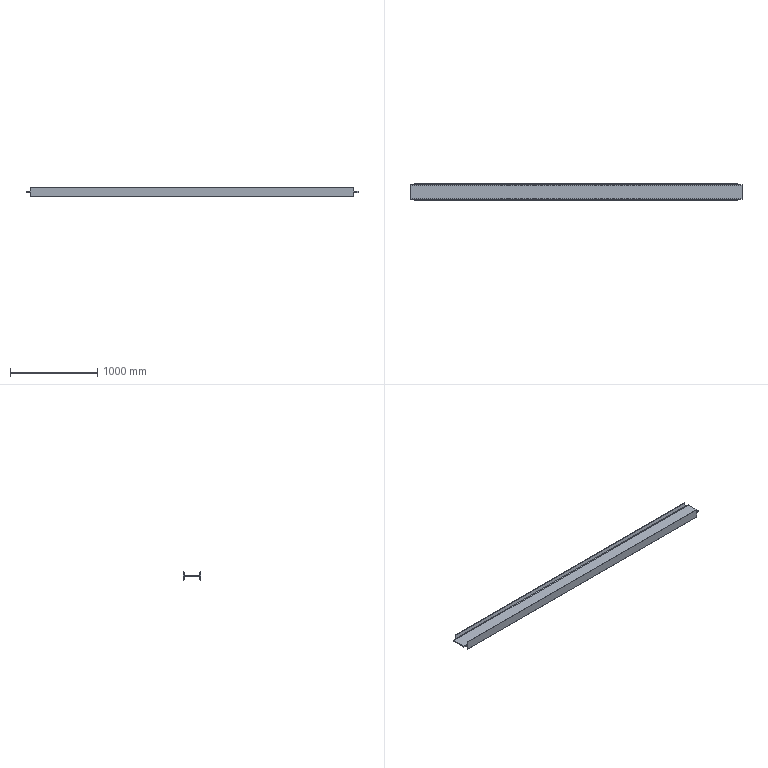Part | SolidWorks | features Fillet 2, ICE 2, Extrusion 1 | 1 solid | 30 faces | box 3800 x 200 x 102 mm | volume 14290911 mm3 | plane 22 | cylinder 8 | commonest cylinder face diameters 9 x4 18 x4
STEP:
#1=CARTESIAN_POINT('',(0.,15.,8.033));
#2=VERTEX_POINT('',#1);
#3=CARTESIAN_POINT('',(0.,15.,-8.033));
#4=VERTEX_POINT('',#3);
#5=CARTESIAN_POINT('',(0.,15.,51.));
#6=DIRECTION('',(0.,0.,-1.));
#7=VECTOR('',#6,1000.);
#8=LINE('',#5,#7);
#9=EDGE_CURVE('',#2,#4,#8,.T.);
#10=ORIENTED_EDGE('',*,*,#9,.F.);
#11=CARTESIAN_POINT('',(0.,22.149,4.5));
#12=VERTEX_POINT('',#11);
#13=CARTESIAN_POINT('',(0.,22.149,13.5));
#14=DIRECTION('',(1.,0.,0.));
#15=DIRECTION('',(0.,0.,-1.));
#16=AXIS2_PLACEMENT_3D('',#13,#14,#15);
#17=CIRCLE('',#16,9.);
#18=EDGE_CURVE('',#2,#12,#17,.T.);
#19=ORIENTED_EDGE('',*,*,#18,.T.);
#20=CARTESIAN_POINT('',(0.,177.851,4.5));
#21=VERTEX_POINT('',#20);
#22=CARTESIAN_POINT('',(0.,185.475,4.5));
#23=DIRECTION('',(0.,-1.,0.));
#24=VECTOR('',#23,1000.);
#25=LINE('',#22,#24);
#26=EDGE_CURVE('',#21,#12,#25,.T.);
#27=ORIENTED_EDGE('',*,*,#26,.F.);
#28=CARTESIAN_POINT('',(0.,185.,8.033));
#29=VERTEX_POINT('',#28);
#30=CARTESIAN_POINT('',(0.,177.851,13.5));
#31=DIRECTION('',(1.,0.,0.));
#32=DIRECTION('',(0.,0.,-1.));
#33=AXIS2_PLACEMENT_3D('',#30,#31,#32);
#34=CIRCLE('',#33,9.);
#35=EDGE_CURVE('',#21,#29,#34,.T.);
#36=ORIENTED_EDGE('',*,*,#35,.T.);
#37=CARTESIAN_POINT('',(0.,185.,-8.033));
#38=VERTEX_POINT('',#37);
#39=CARTESIAN_POINT('',(0.,185.,51.));
#40=DIRECTION('',(0.,0.,1.));
#41=VECTOR('',#40,1000.);
#42=LINE('',#39,#41);
#43=EDGE_CURVE('',#38,#29,#42,.T.);
#44=ORIENTED_EDGE('',*,*,#43,.F.);
#45=CARTESIAN_POINT('',(0.,177.851,-4.5));
#46=VERTEX_POINT('',#45);
#47=CARTESIAN_POINT('',(0.,177.851,-13.5));
#48=DIRECTION('',(1.,0.,0.));
#49=DIRECTION('',(0.,0.,-1.));
#50=AXIS2_PLACEMENT_3D('',#47,#48,#49);
#51=CIRCLE('',#50,9.);
#52=EDGE_CURVE('',#38,#46,#51,.T.);
#53=ORIENTED_EDGE('',*,*,#52,.T.);
#54=CARTESIAN_POINT('',(0.,22.149,-4.5));
#55=VERTEX_POINT('',#54);
#56=CARTESIAN_POINT('',(0.,185.475,-4.5));
#57=DIRECTION('',(0.,1.,0.));
#58=VECTOR('',#57,1000.);
#59=LINE('',#56,#58);
#60=EDGE_CURVE('',#55,#46,#59,.T.);
#61=ORIENTED_EDGE('',*,*,#60,.F.);
#62=CARTESIAN_POINT('',(0.,22.149,-13.5));
#63=DIRECTION('',(1.,0.,0.));
#64=DIRECTION('',(0.,0.,-1.));
#65=AXIS2_PLACEMENT_3D('',#62,#63,#64);
#66=CIRCLE('',#65,9.);
#67=EDGE_CURVE('',#55,#4,#66,.T.);
#68=ORIENTED_EDGE('',*,*,#67,.T.);
#69=EDGE_LOOP('',(#10,#19,#27,#36,#44,#53,#61,#68));
#70=FACE_OUTER_BOUND('',#69,.T.);
#71=CARTESIAN_POINT('',(0.,200.,51.));
#72=DIRECTION('',(1.,0.,0.));
#73=DIRECTION('',(0.,0.,-1.));
#74=AXIS2_PLACEMENT_3D('',#71,#72,#73);
#75=PLANE('',#74);
#76=ADVANCED_FACE('',(#70),#75,.F.);
#77=CARTESIAN_POINT('',(3753.5,2.963,51.));
#78=VERTEX_POINT('',#77);
#79=CARTESIAN_POINT('',(46.5,2.963,51.));
#80=VERTEX_POINT('',#79);
#81=CARTESIAN_POINT('',(3800.,2.963,51.));
#82=DIRECTION('',(-1.,0.,0.));
#83=VECTOR('',#82,1000.);
#84=LINE('',#81,#83);
#85=EDGE_CURVE('',#78,#80,#84,.T.);
#86=ORIENTED_EDGE('',*,*,#85,.T.);
#87=CARTESIAN_POINT('',(46.5,0.,51.));
#88=VERTEX_POINT('',#87);
#89=CARTESIAN_POINT('',(46.5,15.,51.));
#90=DIRECTION('',(0.,-1.,0.));
#91=VECTOR('',#90,1000.);
#92=LINE('',#89,#91);
#93=EDGE_CURVE('',#80,#88,#92,.T.);
#94=ORIENTED_EDGE('',*,*,#93,.T.);
#95=CARTESIAN_POINT('',(3753.5,0.,51.));
#96=VERTEX_POINT('',#95);
#97=CARTESIAN_POINT('',(3800.,0.,51.));
#98=DIRECTION('',(-1.,0.,0.));
#99=VECTOR('',#98,1000.);
#100=LINE('',#97,#99);
#101=EDGE_CURVE('',#96,#88,#100,.T.);
#102=ORIENTED_EDGE('',*,*,#101,.F.);
#103=CARTESIAN_POINT('',(3753.5,15.,51.));
#104=DIRECTION('',(0.,-1.,0.));
#105=VECTOR('',#104,1000.);
#106=LINE('',#103,#105);
#107=EDGE_CURVE('',#78,#96,#106,.T.);
#108=ORIENTED_EDGE('',*,*,#107,.F.);
#109=EDGE_LOOP('',(#86,#94,#102,#108));
#110=FACE_OUTER_BOUND('',#109,.T.);
#111=CARTESIAN_POINT('',(3800.,6.775,51.));
#112=DIRECTION('',(0.,0.,-1.));
#113=DIRECTION('',(-1.,0.,0.));
#114=AXIS2_PLACEMENT_3D('',#111,#112,#113);
#115=PLANE('',#114);
#116=ADVANCED_FACE('',(#110),#115,.F.);
#117=ORIENTED_EDGE('',*,*,#101,.T.);
#118=CARTESIAN_POINT('',(46.5,0.,-51.));
#119=VERTEX_POINT('',#118);
#120=CARTESIAN_POINT('',(46.5,0.,51.));
#121=DIRECTION('',(0.,0.,1.));
#122=VECTOR('',#121,1000.);
#123=LINE('',#120,#122);
#124=EDGE_CURVE('',#119,#88,#123,.T.);
#125=ORIENTED_EDGE('',*,*,#124,.F.);
#126=CARTESIAN_POINT('',(3753.5,0.,-51.));
#127=VERTEX_POINT('',#126);
#128=CARTESIAN_POINT('',(3800.,0.,-51.));
#129=DIRECTION('',(-1.,0.,0.));
#130=VECTOR('',#129,1000.);
#131=LINE('',#128,#130);
#132=EDGE_CURVE('',#127,#119,#131,.T.);
#133=ORIENTED_EDGE('',*,*,#132,.F.);
#134=CARTESIAN_POINT('',(3753.5,0.,51.));
#135=DIRECTION('',(0.,0.,-1.));
#136=VECTOR('',#135,1000.);
#137=LINE('',#134,#136);
#138=EDGE_CURVE('',#96,#127,#137,.T.);
#139=ORIENTED_EDGE('',*,*,#138,.F.);
#140=EDGE_LOOP('',(#117,#125,#133,#139));
#141=FACE_OUTER_BOUND('',#140,.T.);
#142=CARTESIAN_POINT('',(3800.,0.,51.));
#143=DIRECTION('',(0.,1.,0.));
#144=DIRECTION('',(0.,0.,1.));
#145=AXIS2_PLACEMENT_3D('',#142,#143,#144);
#146=PLANE('',#145);
#147=ADVANCED_FACE('',(#141),#146,.F.);
#148=ORIENTED_EDGE('',*,*,#132,.T.);
#149=CARTESIAN_POINT('',(46.5,2.963,-51.));
#150=VERTEX_POINT('',#149);
#151=CARTESIAN_POINT('',(46.5,15.,-51.));
#152=DIRECTION('',(0.,-1.,0.));
#153=VECTOR('',#152,1000.);
#154=LINE('',#151,#153);
#155=EDGE_CURVE('',#150,#119,#154,.T.);
#156=ORIENTED_EDGE('',*,*,#155,.F.);
#157=CARTESIAN_POINT('',(3753.5,2.963,-51.));
#158=VERTEX_POINT('',#157);
#159=CARTESIAN_POINT('',(3800.,2.963,-51.));
#160=DIRECTION('',(1.,0.,0.));
#161=VECTOR('',#160,1000.);
#162=LINE('',#159,#161);
#163=EDGE_CURVE('',#150,#158,#162,.T.);
#164=ORIENTED_EDGE('',*,*,#163,.T.);
#165=CARTESIAN_POINT('',(3753.5,15.,-51.));
#166=DIRECTION('',(0.,-1.,0.));
#167=VECTOR('',#166,1000.);
#168=LINE('',#165,#167);
#169=EDGE_CURVE('',#158,#127,#168,.T.);
#170=ORIENTED_EDGE('',*,*,#169,.T.);
#171=EDGE_LOOP('',(#148,#156,#164,#170));
#172=FACE_OUTER_BOUND('',#171,.T.);
#173=CARTESIAN_POINT('',(3800.,6.775,-51.));
#174=DIRECTION('',(0.,0.,1.));
#175=DIRECTION('',(1.,0.,0.));
#176=AXIS2_PLACEMENT_3D('',#173,#174,#175);
#177=PLANE('',#176);
#178=ADVANCED_FACE('',(#172),#177,.F.);
#179=CARTESIAN_POINT('',(3753.5,7.402,-47.24));
#180=VERTEX_POINT('',#179);
#181=CARTESIAN_POINT('',(46.5,7.402,-47.24));
#182=VERTEX_POINT('',#181);
#183=CARTESIAN_POINT('',(3800.,7.402,-47.24));
#184=DIRECTION('',(-1.,0.,0.));
#185=VECTOR('',#184,1000.);
#186=LINE('',#183,#185);
#187=EDGE_CURVE('',#180,#182,#186,.T.);
#188=ORIENTED_EDGE('',*,*,#187,.T.);
#189=CARTESIAN_POINT('',(46.5,13.272,-12.02));
#190=VERTEX_POINT('',#189);
#191=CARTESIAN_POINT('',(46.5,14.525,-4.5));
#192=DIRECTION('',(0.,0.1644,0.9864));
#193=VECTOR('',#192,1000.);
#194=LINE('',#191,#193);
#195=EDGE_CURVE('',#182,#190,#194,.T.);
#196=ORIENTED_EDGE('',*,*,#195,.T.);
#197=CARTESIAN_POINT('',(3753.5,13.272,-12.02));
#198=VERTEX_POINT('',#197);
#199=CARTESIAN_POINT('',(3800.,13.272,-12.02));
#200=DIRECTION('',(1.,0.,0.));
#201=VECTOR('',#200,1000.);
#202=LINE('',#199,#201);
#203=EDGE_CURVE('',#190,#198,#202,.T.);
#204=ORIENTED_EDGE('',*,*,#203,.T.);
#205=CARTESIAN_POINT('',(3753.5,14.525,-4.5));
#206=DIRECTION('',(0.,-0.1644,-0.9864));
#207=VECTOR('',#206,1000.);
#208=LINE('',#205,#207);
#209=EDGE_CURVE('',#198,#180,#208,.T.);
#210=ORIENTED_EDGE('',*,*,#209,.T.);
#211=EDGE_LOOP('',(#188,#196,#204,#210));
#212=FACE_OUTER_BOUND('',#211,.T.);
#213=CARTESIAN_POINT('',(3800.,14.525,-4.5));
#214=DIRECTION('',(0.,-0.9864,0.1644));
#215=DIRECTION('',(0.,-0.1644,-0.9864));
#216=AXIS2_PLACEMENT_3D('',#213,#214,#215);
#217=PLANE('',#216);
#218=ADVANCED_FACE('',(#212),#217,.F.);
#219=ORIENTED_EDGE('',*,*,#60,.T.);
#220=CARTESIAN_POINT('',(3800.,177.851,-4.5));
#221=VERTEX_POINT('',#220);
#222=CARTESIAN_POINT('',(3800.,177.851,-4.5));
#223=DIRECTION('',(1.,0.,0.));
#224=VECTOR('',#223,1000.);
#225=LINE('',#222,#224);
#226=EDGE_CURVE('',#46,#221,#225,.T.);
#227=ORIENTED_EDGE('',*,*,#226,.T.);
#228=CARTESIAN_POINT('',(3800.,22.149,-4.5));
#229=VERTEX_POINT('',#228);
#230=CARTESIAN_POINT('',(3800.,185.475,-4.5));
#231=DIRECTION('',(0.,1.,0.));
#232=VECTOR('',#231,1000.);
#233=LINE('',#230,#232);
#234=EDGE_CURVE('',#229,#221,#233,.T.);
#235=ORIENTED_EDGE('',*,*,#234,.F.);
#236=CARTESIAN_POINT('',(0.,22.149,-4.5));
#237=DIRECTION('',(-1.,0.,0.));
#238=VECTOR('',#237,1000.);
#239=LINE('',#236,#238);
#240=EDGE_CURVE('',#229,#55,#239,.T.);
#241=ORIENTED_EDGE('',*,*,#240,.T.);
#242=EDGE_LOOP('',(#219,#227,#235,#241));
#243=FACE_OUTER_BOUND('',#242,.T.);
#244=CARTESIAN_POINT('',(3800.,185.475,-4.5));
#245=DIRECTION('',(0.,0.,1.));
#246=DIRECTION('',(0.,-1.,0.));
#247=AXIS2_PLACEMENT_3D('',#244,#245,#246);
#248=PLANE('',#247);
#249=ADVANCED_FACE('',(#243),#248,.F.);
#250=CARTESIAN_POINT('',(3753.5,186.728,-12.02));
#251=VERTEX_POINT('',#250);
#252=CARTESIAN_POINT('',(46.5,186.728,-12.02));
#253=VERTEX_POINT('',#252);
#254=CARTESIAN_POINT('',(0.,186.728,-12.02));
#255=DIRECTION('',(-1.,0.,0.));
#256=VECTOR('',#255,1000.);
#257=LINE('',#254,#256);
#258=EDGE_CURVE('',#251,#253,#257,.T.);
#259=ORIENTED_EDGE('',*,*,#258,.T.);
#260=CARTESIAN_POINT('',(46.5,192.598,-47.24));
#261=VERTEX_POINT('',#260);
#262=CARTESIAN_POINT('',(46.5,193.225,-51.));
#263=DIRECTION('',(0.,0.1644,-0.9864));
#264=VECTOR('',#263,1000.);
#265=LINE('',#262,#264);
#266=EDGE_CURVE('',#253,#261,#265,.T.);
#267=ORIENTED_EDGE('',*,*,#266,.T.);
#268=CARTESIAN_POINT('',(3753.5,192.598,-47.24));
#269=VERTEX_POINT('',#268);
#270=CARTESIAN_POINT('',(3800.,192.598,-47.24));
#271=DIRECTION('',(1.,0.,0.));
#272=VECTOR('',#271,1000.);
#273=LINE('',#270,#272);
#274=EDGE_CURVE('',#261,#269,#273,.T.);
#275=ORIENTED_EDGE('',*,*,#274,.T.);
#276=CARTESIAN_POINT('',(3753.5,193.225,-51.));
#277=DIRECTION('',(0.,-0.1644,0.9864));
#278=VECTOR('',#277,1000.);
#279=LINE('',#276,#278);
#280=EDGE_CURVE('',#269,#251,#279,.T.);
#281=ORIENTED_EDGE('',*,*,#280,.T.);
#282=EDGE_LOOP('',(#259,#267,#275,#281));
#283=FACE_OUTER_BOUND('',#282,.T.);
#284=CARTESIAN_POINT('',(3800.,193.225,-51.));
#285=DIRECTION('',(0.,0.9864,0.1644));
#286=DIRECTION('',(0.,-0.1644,0.9864));
#287=AXIS2_PLACEMENT_3D('',#284,#285,#286);
#288=PLANE('',#287);
#289=ADVANCED_FACE('',(#283),#288,.F.);
#290=CARTESIAN_POINT('',(3753.5,197.037,-51.));
#291=VERTEX_POINT('',#290);
#292=CARTESIAN_POINT('',(46.5,197.037,-51.));
#293=VERTEX_POINT('',#292);
#294=CARTESIAN_POINT('',(3800.,197.037,-51.));
#295=DIRECTION('',(-1.,0.,0.));
#296=VECTOR('',#295,1000.);
#297=LINE('',#294,#296);
#298=EDGE_CURVE('',#291,#293,#297,.T.);
#299=ORIENTED_EDGE('',*,*,#298,.T.);
#300=CARTESIAN_POINT('',(46.5,200.,-51.));
#301=VERTEX_POINT('',#300);
#302=CARTESIAN_POINT('',(46.5,185.,-51.));
#303=DIRECTION('',(0.,1.,0.));
#304=VECTOR('',#303,1000.);
#305=LINE('',#302,#304);
#306=EDGE_CURVE('',#293,#301,#305,.T.);
#307=ORIENTED_EDGE('',*,*,#306,.T.);
#308=CARTESIAN_POINT('',(3753.5,200.,-51.));
#309=VERTEX_POINT('',#308);
#310=CARTESIAN_POINT('',(3800.,200.,-51.));
#311=DIRECTION('',(-1.,0.,0.));
#312=VECTOR('',#311,1000.);
#313=LINE('',#310,#312);
#314=EDGE_CURVE('',#309,#301,#313,.T.);
#315=ORIENTED_EDGE('',*,*,#314,.F.);
#316=CARTESIAN_POINT('',(3753.5,185.,-51.));
#317=DIRECTION('',(0.,1.,0.));
#318=VECTOR('',#317,1000.);
#319=LINE('',#316,#318);
#320=EDGE_CURVE('',#291,#309,#319,.T.);
#321=ORIENTED_EDGE('',*,*,#320,.F.);
#322=EDGE_LOOP('',(#299,#307,#315,#321));
#323=FACE_OUTER_BOUND('',#322,.T.);
#324=CARTESIAN_POINT('',(3800.,200.,-51.));
#325=DIRECTION('',(0.,0.,1.));
#326=DIRECTION('',(0.,-1.,0.));
#327=AXIS2_PLACEMENT_3D('',#324,#325,#326);
#328=PLANE('',#327);
#329=ADVANCED_FACE('',(#323),#328,.F.);
#330=ORIENTED_EDGE('',*,*,#314,.T.);
#331=CARTESIAN_POINT('',(46.5,200.,51.));
#332=VERTEX_POINT('',#331);
#333=CARTESIAN_POINT('',(46.5,200.,51.));
#334=DIRECTION('',(0.,0.,-1.));
#335=VECTOR('',#334,1000.);
#336=LINE('',#333,#335);
#337=EDGE_CURVE('',#332,#301,#336,.T.);
#338=ORIENTED_EDGE('',*,*,#337,.F.);
#339=CARTESIAN_POINT('',(3753.5,200.,51.));
#340=VERTEX_POINT('',#339);
#341=CARTESIAN_POINT('',(3800.,200.,51.));
#342=DIRECTION('',(-1.,0.,0.));
#343=VECTOR('',#342,1000.);
#344=LINE('',#341,#343);
#345=EDGE_CURVE('',#340,#332,#344,.T.);
#346=ORIENTED_EDGE('',*,*,#345,.F.);
#347=CARTESIAN_POINT('',(3753.5,200.,-51.));
#348=DIRECTION('',(0.,0.,1.));
#349=VECTOR('',#348,1000.);
#350=LINE('',#347,#349);
#351=EDGE_CURVE('',#309,#340,#350,.T.);
#352=ORIENTED_EDGE('',*,*,#351,.F.);
#353=EDGE_LOOP('',(#330,#338,#346,#352));
#354=FACE_OUTER_BOUND('',#353,.T.);
#355=CARTESIAN_POINT('',(3800.,200.,51.));
#356=DIRECTION('',(0.,-1.,0.));
#357=DIRECTION('',(0.,0.,-1.));
#358=AXIS2_PLACEMENT_3D('',#355,#356,#357);
#359=PLANE('',#358);
#360=ADVANCED_FACE('',(#354),#359,.F.);
#361=ORIENTED_EDGE('',*,*,#345,.T.);
#362=CARTESIAN_POINT('',(46.5,197.037,51.));
#363=VERTEX_POINT('',#362);
#364=CARTESIAN_POINT('',(46.5,185.,51.));
#365=DIRECTION('',(0.,1.,0.));
#366=VECTOR('',#365,1000.);
#367=LINE('',#364,#366);
#368=EDGE_CURVE('',#363,#332,#367,.T.);
#369=ORIENTED_EDGE('',*,*,#368,.F.);
#370=CARTESIAN_POINT('',(3753.5,197.037,51.));
#371=VERTEX_POINT('',#370);
#372=CARTESIAN_POINT('',(3800.,197.037,51.));
#373=DIRECTION('',(1.,0.,0.));
#374=VECTOR('',#373,1000.);
#375=LINE('',#372,#374);
#376=EDGE_CURVE('',#363,#371,#375,.T.);
#377=ORIENTED_EDGE('',*,*,#376,.T.);
#378=CARTESIAN_POINT('',(3753.5,185.,51.));
#379=DIRECTION('',(0.,1.,0.));
#380=VECTOR('',#379,1000.);
#381=LINE('',#378,#380);
#382=EDGE_CURVE('',#371,#340,#381,.T.);
#383=ORIENTED_EDGE('',*,*,#382,.T.);
#384=EDGE_LOOP('',(#361,#369,#377,#383));
#385=FACE_OUTER_BOUND('',#384,.T.);
#386=CARTESIAN_POINT('',(3800.,200.,51.));
#387=DIRECTION('',(0.,0.,-1.));
#388=DIRECTION('',(0.,1.,0.));
#389=AXIS2_PLACEMENT_3D('',#386,#387,#388);
#390=PLANE('',#389);
#391=ADVANCED_FACE('',(#385),#390,.F.);
#392=CARTESIAN_POINT('',(3753.5,192.598,47.24));
#393=VERTEX_POINT('',#392);
#394=CARTESIAN_POINT('',(46.5,192.598,47.24));
#395=VERTEX_POINT('',#394);
#396=CARTESIAN_POINT('',(3800.,192.598,47.24));
#397=DIRECTION('',(-1.,0.,0.));
#398=VECTOR('',#397,1000.);
#399=LINE('',#396,#398);
#400=EDGE_CURVE('',#393,#395,#399,.T.);
#401=ORIENTED_EDGE('',*,*,#400,.T.);
#402=CARTESIAN_POINT('',(46.5,186.728,12.02));
#403=VERTEX_POINT('',#402);
#404=CARTESIAN_POINT('',(46.5,193.225,51.));
#405=DIRECTION('',(0.,-0.1644,-0.9864));
#406=VECTOR('',#405,1000.);
#407=LINE('',#404,#406);
#408=EDGE_CURVE('',#395,#403,#407,.T.);
#409=ORIENTED_EDGE('',*,*,#408,.T.);
#410=CARTESIAN_POINT('',(3753.5,186.728,12.02));
#411=VERTEX_POINT('',#410);
#412=CARTESIAN_POINT('',(3800.,186.728,12.02));
#413=DIRECTION('',(1.,0.,0.));
#414=VECTOR('',#413,1000.);
#415=LINE('',#412,#414);
#416=EDGE_CURVE('',#403,#411,#415,.T.);
#417=ORIENTED_EDGE('',*,*,#416,.T.);
#418=CARTESIAN_POINT('',(3753.5,193.225,51.));
#419=DIRECTION('',(0.,0.1644,0.9864));
#420=VECTOR('',#419,1000.);
#421=LINE('',#418,#420);
#422=EDGE_CURVE('',#411,#393,#421,.T.);
#423=ORIENTED_EDGE('',*,*,#422,.T.);
#424=EDGE_LOOP('',(#401,#409,#417,#423));
#425=FACE_OUTER_BOUND('',#424,.T.);
#426=CARTESIAN_POINT('',(3800.,193.225,51.));
#427=DIRECTION('',(0.,0.9864,-0.1644));
#428=DIRECTION('',(0.,0.1644,0.9864));
#429=AXIS2_PLACEMENT_3D('',#426,#427,#428);
#430=PLANE('',#429);
#431=ADVANCED_FACE('',(#425),#430,.F.);
#432=ORIENTED_EDGE('',*,*,#26,.T.);
#433=CARTESIAN_POINT('',(3800.,22.149,4.5));
#434=VERTEX_POINT('',#433);
#435=CARTESIAN_POINT('',(3800.,22.149,4.5));
#436=DIRECTION('',(1.,0.,0.));
#437=VECTOR('',#436,1000.);
#438=LINE('',#435,#437);
#439=EDGE_CURVE('',#12,#434,#438,.T.);
#440=ORIENTED_EDGE('',*,*,#439,.T.);
#441=CARTESIAN_POINT('',(3800.,177.851,4.5));
#442=VERTEX_POINT('',#441);
#443=CARTESIAN_POINT('',(3800.,185.475,4.5));
#444=DIRECTION('',(0.,-1.,0.));
#445=VECTOR('',#444,1000.);
#446=LINE('',#443,#445);
#447=EDGE_CURVE('',#442,#434,#446,.T.);
#448=ORIENTED_EDGE('',*,*,#447,.F.);
#449=CARTESIAN_POINT('',(0.,177.851,4.5));
#450=DIRECTION('',(-1.,0.,0.));
#451=VECTOR('',#450,1000.);
#452=LINE('',#449,#451);
#453=EDGE_CURVE('',#442,#21,#452,.T.);
#454=ORIENTED_EDGE('',*,*,#453,.T.);
#455=EDGE_LOOP('',(#432,#440,#448,#454));
#456=FACE_OUTER_BOUND('',#455,.T.);
#457=CARTESIAN_POINT('',(3800.,185.475,4.5));
#458=DIRECTION('',(0.,0.,-1.));
#459=DIRECTION('',(0.,1.,0.));
#460=AXIS2_PLACEMENT_3D('',#457,#458,#459);
#461=PLANE('',#460);
#462=ADVANCED_FACE('',(#456),#461,.F.);
#463=CARTESIAN_POINT('',(3753.5,13.272,12.02));
#464=VERTEX_POINT('',#463);
#465=CARTESIAN_POINT('',(46.5,13.272,12.02));
#466=VERTEX_POINT('',#465);
#467=CARTESIAN_POINT('',(0.,13.272,12.02));
#468=DIRECTION('',(-1.,0.,0.));
#469=VECTOR('',#468,1000.);
#470=LINE('',#467,#469);
#471=EDGE_CURVE('',#464,#466,#470,.T.);
#472=ORIENTED_EDGE('',*,*,#471,.T.);
#473=CARTESIAN_POINT('',(46.5,7.402,47.24));
#474=VERTEX_POINT('',#473);
#475=CARTESIAN_POINT('',(46.5,14.525,4.5));
#476=DIRECTION('',(0.,-0.1644,0.9864));
#477=VECTOR('',#476,1000.);
#478=LINE('',#475,#477);
#479=EDGE_CURVE('',#466,#474,#478,.T.);
#480=ORIENTED_EDGE('',*,*,#479,.T.);
#481=CARTESIAN_POINT('',(3753.5,7.402,47.24));
#482=VERTEX_POINT('',#481);
#483=CARTESIAN_POINT('',(3800.,7.402,47.24));
#484=DIRECTION('',(1.,0.,0.));
#485=VECTOR('',#484,1000.);
#486=LINE('',#483,#485);
#487=EDGE_CURVE('',#474,#482,#486,.T.);
#488=ORIENTED_EDGE('',*,*,#487,.T.);
#489=CARTESIAN_POINT('',(3753.5,14.525,4.5));
#490=DIRECTION('',(0.,0.1644,-0.9864));
#491=VECTOR('',#490,1000.);
#492=LINE('',#489,#491);
#493=EDGE_CURVE('',#482,#464,#492,.T.);
#494=ORIENTED_EDGE('',*,*,#493,.T.);
#495=EDGE_LOOP('',(#472,#480,#488,#494));
#496=FACE_OUTER_BOUND('',#495,.T.);
#497=CARTESIAN_POINT('',(3800.,14.525,4.5));
#498=DIRECTION('',(0.,-0.9864,-0.1644));
#499=DIRECTION('',(0.,0.1644,-0.9864));
#500=AXIS2_PLACEMENT_3D('',#497,#498,#499);
#501=PLANE('',#500);
#502=ADVANCED_FACE('',(#496),#501,.F.);
#503=CARTESIAN_POINT('',(3800.,15.,-8.033));
#504=VERTEX_POINT('',#503);
#505=CARTESIAN_POINT('',(3800.,15.,8.033));
#506=VERTEX_POINT('',#505);
#507=CARTESIAN_POINT('',(3800.,15.,51.));
#508=DIRECTION('',(0.,0.,1.));
#509=VECTOR('',#508,1000.);
#510=LINE('',#507,#509);
#511=EDGE_CURVE('',#504,#506,#510,.T.);
#512=ORIENTED_EDGE('',*,*,#511,.F.);
#513=CARTESIAN_POINT('',(3800.,22.149,-13.5));
#514=DIRECTION('',(-1.,0.,0.));
#515=DIRECTION('',(0.,0.,-1.));
#516=AXIS2_PLACEMENT_3D('',#513,#514,#515);
#517=CIRCLE('',#516,9.);
#518=EDGE_CURVE('',#504,#229,#517,.T.);
#519=ORIENTED_EDGE('',*,*,#518,.T.);
#520=ORIENTED_EDGE('',*,*,#234,.T.);
#521=CARTESIAN_POINT('',(3800.,185.,-8.033));
#522=VERTEX_POINT('',#521);
#523=CARTESIAN_POINT('',(3800.,177.851,-13.5));
#524=DIRECTION('',(-1.,0.,0.));
#525=DIRECTION('',(0.,0.,-1.));
#526=AXIS2_PLACEMENT_3D('',#523,#524,#525);
#527=CIRCLE('',#526,9.);
#528=EDGE_CURVE('',#221,#522,#527,.T.);
#529=ORIENTED_EDGE('',*,*,#528,.T.);
#530=CARTESIAN_POINT('',(3800.,185.,8.033));
#531=VERTEX_POINT('',#530);
#532=CARTESIAN_POINT('',(3800.,185.,-51.));
#533=DIRECTION('',(0.,0.,-1.));
#534=VECTOR('',#533,1000.);
#535=LINE('',#532,#534);
#536=EDGE_CURVE('',#531,#522,#535,.T.);
#537=ORIENTED_EDGE('',*,*,#536,.F.);
#538=CARTESIAN_POINT('',(3800.,177.851,13.5));
#539=DIRECTION('',(-1.,0.,0.));
#540=DIRECTION('',(0.,0.,-1.));
#541=AXIS2_PLACEMENT_3D('',#538,#539,#540);
#542=CIRCLE('',#541,9.);
#543=EDGE_CURVE('',#531,#442,#542,.T.);
#544=ORIENTED_EDGE('',*,*,#543,.T.);
#545=ORIENTED_EDGE('',*,*,#447,.T.);
#546=CARTESIAN_POINT('',(3800.,22.149,13.5));
#547=DIRECTION('',(-1.,0.,0.));
#548=DIRECTION('',(0.,0.,-1.));
#549=AXIS2_PLACEMENT_3D('',#546,#547,#548);
#550=CIRCLE('',#549,9.);
#551=EDGE_CURVE('',#434,#506,#550,.T.);
#552=ORIENTED_EDGE('',*,*,#551,.T.);
#553=EDGE_LOOP('',(#512,#519,#520,#529,#537,#544,#545,#552));
#554=FACE_OUTER_BOUND('',#553,.T.);
#555=CARTESIAN_POINT('',(3800.,200.,51.));
#556=DIRECTION('',(1.,0.,0.));
#557=DIRECTION('',(0.,0.,-1.));
#558=AXIS2_PLACEMENT_3D('',#555,#556,#557);
#559=PLANE('',#558);
#560=ADVANCED_FACE('',(#554),#559,.T.);
#561=CARTESIAN_POINT('',(46.5,185.,-8.033));
#562=VERTEX_POINT('',#561);
#563=CARTESIAN_POINT('',(3800.,185.,-8.033));
#564=DIRECTION('',(1.,0.,0.));
#565=VECTOR('',#564,1000.);
#566=LINE('',#563,#565);
#567=EDGE_CURVE('',#38,#562,#566,.T.);
#568=ORIENTED_EDGE('',*,*,#567,.T.);
#569=CARTESIAN_POINT('',(46.5,177.851,-13.5));
#570=DIRECTION('',(-1.,0.,0.));
#571=DIRECTION('',(0.,0.,-1.));
#572=AXIS2_PLACEMENT_3D('',#569,#570,#571);
#573=CIRCLE('',#572,9.);
#574=EDGE_CURVE('',#562,#253,#573,.T.);
#575=ORIENTED_EDGE('',*,*,#574,.T.);
#576=ORIENTED_EDGE('',*,*,#258,.F.);
#577=CARTESIAN_POINT('',(3753.5,185.,-8.033));
#578=VERTEX_POINT('',#577);
#579=CARTESIAN_POINT('',(3753.5,177.851,-13.5));
#580=DIRECTION('',(1.,0.,0.));
#581=DIRECTION('',(0.,0.,1.));
#582=AXIS2_PLACEMENT_3D('',#579,#580,#581);
#583=CIRCLE('',#582,9.);
#584=EDGE_CURVE('',#251,#578,#583,.T.);
#585=ORIENTED_EDGE('',*,*,#584,.T.);
#586=CARTESIAN_POINT('',(3800.,185.,-8.033));
#587=DIRECTION('',(1.,0.,0.));
#588=VECTOR('',#587,1000.);
#589=LINE('',#586,#588);
#590=EDGE_CURVE('',#578,#522,#589,.T.);
#591=ORIENTED_EDGE('',*,*,#590,.T.);
#592=ORIENTED_EDGE('',*,*,#528,.F.);
#593=ORIENTED_EDGE('',*,*,#226,.F.);
#594=ORIENTED_EDGE('',*,*,#52,.F.);
#595=EDGE_LOOP('',(#568,#575,#576,#585,#591,#592,#593,#594));
#596=FACE_OUTER_BOUND('',#595,.T.);
#597=CARTESIAN_POINT('',(3800.,177.851,-13.5));
#598=DIRECTION('',(1.,0.,0.));
#599=DIRECTION('',(0.,0.,-1.));
#600=AXIS2_PLACEMENT_3D('',#597,#598,#599);
#601=CYLINDRICAL_SURFACE('',#600,9.);
#602=ADVANCED_FACE('',(#596),#601,.F.);
#603=ORIENTED_EDGE('',*,*,#203,.F.);
#604=CARTESIAN_POINT('',(46.5,15.,-8.033));
#605=VERTEX_POINT('',#604);
#606=CARTESIAN_POINT('',(46.5,22.149,-13.5));
#607=DIRECTION('',(-1.,0.,0.));
#608=DIRECTION('',(0.,0.,-1.));
#609=AXIS2_PLACEMENT_3D('',#606,#607,#608);
#610=CIRCLE('',#609,9.);
#611=EDGE_CURVE('',#190,#605,#610,.T.);
#612=ORIENTED_EDGE('',*,*,#611,.T.);
#613=CARTESIAN_POINT('',(3800.,15.,-8.033));
#614=DIRECTION('',(1.,0.,0.));
#615=VECTOR('',#614,1000.);
#616=LINE('',#613,#615);
#617=EDGE_CURVE('',#4,#605,#616,.T.);
#618=ORIENTED_EDGE('',*,*,#617,.F.);
#619=ORIENTED_EDGE('',*,*,#67,.F.);
#620=ORIENTED_EDGE('',*,*,#240,.F.);
#621=ORIENTED_EDGE('',*,*,#518,.F.);
#622=CARTESIAN_POINT('',(3753.5,15.,-8.033));
#623=VERTEX_POINT('',#622);
#624=CARTESIAN_POINT('',(3800.,15.,-8.033));
#625=DIRECTION('',(-1.,0.,0.));
#626=VECTOR('',#625,1000.);
#627=LINE('',#624,#626);
#628=EDGE_CURVE('',#504,#623,#627,.T.);
#629=ORIENTED_EDGE('',*,*,#628,.T.);
#630=CARTESIAN_POINT('',(3753.5,22.149,-13.5));
#631=DIRECTION('',(1.,0.,0.));
#632=DIRECTION('',(0.,0.,1.));
#633=AXIS2_PLACEMENT_3D('',#630,#631,#632);
#634=CIRCLE('',#633,9.);
#635=EDGE_CURVE('',#623,#198,#634,.T.);
#636=ORIENTED_EDGE('',*,*,#635,.T.);
#637=EDGE_LOOP('',(#603,#612,#618,#619,#620,#621,#629,#636));
#638=FACE_OUTER_BOUND('',#637,.T.);
#639=CARTESIAN_POINT('',(3800.,22.149,-13.5));
#640=DIRECTION('',(1.,0.,0.));
#641=DIRECTION('',(0.,0.,-1.));
#642=AXIS2_PLACEMENT_3D('',#639,#640,#641);
#643=CYLINDRICAL_SURFACE('',#642,9.);
#644=ADVANCED_FACE('',(#638),#643,.F.);
#645=CARTESIAN_POINT('',(46.5,15.,8.033));
#646=VERTEX_POINT('',#645);
#647=CARTESIAN_POINT('',(3800.,15.,8.033));
#648=DIRECTION('',(-1.,0.,0.));
#649=VECTOR('',#648,1000.);
#650=LINE('',#647,#649);
#651=EDGE_CURVE('',#646,#2,#650,.T.);
#652=ORIENTED_EDGE('',*,*,#651,.F.);
#653=CARTESIAN_POINT('',(46.5,22.149,13.5));
#654=DIRECTION('',(-1.,0.,0.));
#655=DIRECTION('',(0.,0.,-1.));
#656=AXIS2_PLACEMENT_3D('',#653,#654,#655);
#657=CIRCLE('',#656,9.);
#658=EDGE_CURVE('',#646,#466,#657,.T.);
#659=ORIENTED_EDGE('',*,*,#658,.T.);
#660=ORIENTED_EDGE('',*,*,#471,.F.);
#661=CARTESIAN_POINT('',(3753.5,15.,8.033));
#662=VERTEX_POINT('',#661);
#663=CARTESIAN_POINT('',(3753.5,22.149,13.5));
#664=DIRECTION('',(1.,0.,0.));
#665=DIRECTION('',(0.,0.,1.));
#666=AXIS2_PLACEMENT_3D('',#663,#664,#665);
#667=CIRCLE('',#666,9.);
#668=EDGE_CURVE('',#464,#662,#667,.T.);
#669=ORIENTED_EDGE('',*,*,#668,.T.);
#670=CARTESIAN_POINT('',(3800.,15.,8.033));
#671=DIRECTION('',(1.,0.,0.));
#672=VECTOR('',#671,1000.);
#673=LINE('',#670,#672);
#674=EDGE_CURVE('',#662,#506,#673,.T.);
#675=ORIENTED_EDGE('',*,*,#674,.T.);
#676=ORIENTED_EDGE('',*,*,#551,.F.);
#677=ORIENTED_EDGE('',*,*,#439,.F.);
#678=ORIENTED_EDGE('',*,*,#18,.F.);
#679=EDGE_LOOP('',(#652,#659,#660,#669,#675,#676,#677,#678));
#680=FACE_OUTER_BOUND('',#679,.T.);
#681=CARTESIAN_POINT('',(3800.,22.149,13.5));
#682=DIRECTION('',(1.,0.,0.));
#683=DIRECTION('',(0.,0.,-1.));
#684=AXIS2_PLACEMENT_3D('',#681,#682,#683);
#685=CYLINDRICAL_SURFACE('',#684,9.);
#686=ADVANCED_FACE('',(#680),#685,.F.);
#687=ORIENTED_EDGE('',*,*,#416,.F.);
#688=CARTESIAN_POINT('',(46.5,185.,8.033));
#689=VERTEX_POINT('',#688);
#690=CARTESIAN_POINT('',(46.5,177.851,13.5));
#691=DIRECTION('',(-1.,0.,0.));
#692=DIRECTION('',(0.,0.,-1.));
#693=AXIS2_PLACEMENT_3D('',#690,#691,#692);
#694=CIRCLE('',#693,9.);
#695=EDGE_CURVE('',#403,#689,#694,.T.);
#696=ORIENTED_EDGE('',*,*,#695,.T.);
#697=CARTESIAN_POINT('',(3800.,185.,8.033));
#698=DIRECTION('',(-1.,0.,0.));
#699=VECTOR('',#698,1000.);
#700=LINE('',#697,#699);
#701=EDGE_CURVE('',#689,#29,#700,.T.);
#702=ORIENTED_EDGE('',*,*,#701,.T.);
#703=ORIENTED_EDGE('',*,*,#35,.F.);
#704=ORIENTED_EDGE('',*,*,#453,.F.);
#705=ORIENTED_EDGE('',*,*,#543,.F.);
#706=CARTESIAN_POINT('',(3753.5,185.,8.033));
#707=VERTEX_POINT('',#706);
#708=CARTESIAN_POINT('',(3800.,185.,8.033));
#709=DIRECTION('',(-1.,0.,0.));
#710=VECTOR('',#709,1000.);
#711=LINE('',#708,#710);
#712=EDGE_CURVE('',#531,#707,#711,.T.);
#713=ORIENTED_EDGE('',*,*,#712,.T.);
#714=CARTESIAN_POINT('',(3753.5,177.851,13.5));
#715=DIRECTION('',(1.,0.,0.));
#716=DIRECTION('',(0.,0.,1.));
#717=AXIS2_PLACEMENT_3D('',#714,#715,#716);
#718=CIRCLE('',#717,9.);
#719=EDGE_CURVE('',#707,#411,#718,.T.);
#720=ORIENTED_EDGE('',*,*,#719,.T.);
#721=EDGE_LOOP('',(#687,#696,#702,#703,#704,#705,#713,#720));
#722=FACE_OUTER_BOUND('',#721,.T.);
#723=CARTESIAN_POINT('',(3800.,177.851,13.5));
#724=DIRECTION('',(1.,0.,0.));
#725=DIRECTION('',(0.,0.,-1.));
#726=AXIS2_PLACEMENT_3D('',#723,#724,#725);
#727=CYLINDRICAL_SURFACE('',#726,9.);
#728=ADVANCED_FACE('',(#722),#727,.F.);
#729=CARTESIAN_POINT('',(46.5,197.037,46.5));
#730=DIRECTION('',(-1.,0.,0.));
#731=DIRECTION('',(0.,0.,-1.));
#732=AXIS2_PLACEMENT_3D('',#729,#730,#731);
#733=CIRCLE('',#732,4.5);
#734=EDGE_CURVE('',#395,#363,#733,.T.);
#735=ORIENTED_EDGE('',*,*,#734,.F.);
#736=ORIENTED_EDGE('',*,*,#400,.F.);
#737=CARTESIAN_POINT('',(3753.5,197.037,46.5));
#738=DIRECTION('',(1.,0.,0.));
#739=DIRECTION('',(0.,0.,1.));
#740=AXIS2_PLACEMENT_3D('',#737,#738,#739);
#741=CIRCLE('',#740,4.5);
#742=EDGE_CURVE('',#371,#393,#741,.T.);
#743=ORIENTED_EDGE('',*,*,#742,.F.);
#744=ORIENTED_EDGE('',*,*,#376,.F.);
#745=EDGE_LOOP('',(#735,#736,#743,#744));
#746=FACE_OUTER_BOUND('',#745,.T.);
#747=CARTESIAN_POINT('',(3800.,197.037,46.5));
#748=DIRECTION('',(-1.,0.,0.));
#749=DIRECTION('',(0.,0.,1.));
#750=AXIS2_PLACEMENT_3D('',#747,#748,#749);
#751=CYLINDRICAL_SURFACE('',#750,4.5);
#752=ADVANCED_FACE('',(#746),#751,.T.);
#753=CARTESIAN_POINT('',(46.5,2.963,46.5));
#754=DIRECTION('',(-1.,0.,0.));
#755=DIRECTION('',(0.,0.,-1.));
#756=AXIS2_PLACEMENT_3D('',#753,#754,#755);
#757=CIRCLE('',#756,4.5);
#758=EDGE_CURVE('',#80,#474,#757,.T.);
#759=ORIENTED_EDGE('',*,*,#758,.F.);
#760=ORIENTED_EDGE('',*,*,#85,.F.);
#761=CARTESIAN_POINT('',(3753.5,2.963,46.5));
#762=DIRECTION('',(1.,0.,0.));
#763=DIRECTION('',(0.,0.,1.));
#764=AXIS2_PLACEMENT_3D('',#761,#762,#763);
#765=CIRCLE('',#764,4.5);
#766=EDGE_CURVE('',#482,#78,#765,.T.);
#767=ORIENTED_EDGE('',*,*,#766,.F.);
#768=ORIENTED_EDGE('',*,*,#487,.F.);
#769=EDGE_LOOP('',(#759,#760,#767,#768));
#770=FACE_OUTER_BOUND('',#769,.T.);
#771=CARTESIAN_POINT('',(3800.,2.963,46.5));
#772=DIRECTION('',(-1.,0.,0.));
#773=DIRECTION('',(0.,0.,1.));
#774=AXIS2_PLACEMENT_3D('',#771,#772,#773);
#775=CYLINDRICAL_SURFACE('',#774,4.5);
#776=ADVANCED_FACE('',(#770),#775,.T.);
#777=CARTESIAN_POINT('',(46.5,2.963,-46.5));
#778=DIRECTION('',(-1.,0.,0.));
#779=DIRECTION('',(0.,0.,-1.));
#780=AXIS2_PLACEMENT_3D('',#777,#778,#779);
#781=CIRCLE('',#780,4.5);
#782=EDGE_CURVE('',#182,#150,#781,.T.);
#783=ORIENTED_EDGE('',*,*,#782,.F.);
#784=ORIENTED_EDGE('',*,*,#187,.F.);
#785=CARTESIAN_POINT('',(3753.5,2.963,-46.5));
#786=DIRECTION('',(1.,0.,0.));
#787=DIRECTION('',(0.,0.,1.));
#788=AXIS2_PLACEMENT_3D('',#785,#786,#787);
#789=CIRCLE('',#788,4.5);
#790=EDGE_CURVE('',#158,#180,#789,.T.);
#791=ORIENTED_EDGE('',*,*,#790,.F.);
#792=ORIENTED_EDGE('',*,*,#163,.F.);
#793=EDGE_LOOP('',(#783,#784,#791,#792));
#794=FACE_OUTER_BOUND('',#793,.T.);
#795=CARTESIAN_POINT('',(3800.,2.963,-46.5));
#796=DIRECTION('',(-1.,0.,0.));
#797=DIRECTION('',(0.,0.,1.));
#798=AXIS2_PLACEMENT_3D('',#795,#796,#797);
#799=CYLINDRICAL_SURFACE('',#798,4.5);
#800=ADVANCED_FACE('',(#794),#799,.T.);
#801=CARTESIAN_POINT('',(46.5,197.037,-46.5));
#802=DIRECTION('',(-1.,0.,0.));
#803=DIRECTION('',(0.,0.,-1.));
#804=AXIS2_PLACEMENT_3D('',#801,#802,#803);
#805=CIRCLE('',#804,4.5);
#806=EDGE_CURVE('',#293,#261,#805,.T.);
#807=ORIENTED_EDGE('',*,*,#806,.F.);
#808=ORIENTED_EDGE('',*,*,#298,.F.);
#809=CARTESIAN_POINT('',(3753.5,197.037,-46.5));
#810=DIRECTION('',(1.,0.,0.));
#811=DIRECTION('',(0.,0.,1.));
#812=AXIS2_PLACEMENT_3D('',#809,#810,#811);
#813=CIRCLE('',#812,4.5);
#814=EDGE_CURVE('',#269,#291,#813,.T.);
#815=ORIENTED_EDGE('',*,*,#814,.F.);
#816=ORIENTED_EDGE('',*,*,#274,.F.);
#817=EDGE_LOOP('',(#807,#808,#815,#816));
#818=FACE_OUTER_BOUND('',#817,.T.);
#819=CARTESIAN_POINT('',(3800.,197.037,-46.5));
#820=DIRECTION('',(-1.,0.,0.));
#821=DIRECTION('',(0.,0.,1.));
#822=AXIS2_PLACEMENT_3D('',#819,#820,#821);
#823=CYLINDRICAL_SURFACE('',#822,4.5);
#824=ADVANCED_FACE('',(#818),#823,.T.);
#825=CARTESIAN_POINT('',(3753.5,185.,-51.));
#826=DIRECTION('',(0.,0.,1.));
#827=VECTOR('',#826,1000.);
#828=LINE('',#825,#827);
#829=EDGE_CURVE('',#578,#707,#828,.T.);
#830=ORIENTED_EDGE('',*,*,#829,.T.);
#831=ORIENTED_EDGE('',*,*,#712,.F.);
#832=ORIENTED_EDGE('',*,*,#536,.T.);
#833=ORIENTED_EDGE('',*,*,#590,.F.);
#834=EDGE_LOOP('',(#830,#831,#832,#833));
#835=FACE_OUTER_BOUND('',#834,.T.);
#836=CARTESIAN_POINT('',(0.,185.,0.));
#837=DIRECTION('',(0.,-1.,0.));
#838=DIRECTION('',(0.,0.,-1.));
#839=AXIS2_PLACEMENT_3D('',#836,#837,#838);
#840=PLANE('',#839);
#841=ADVANCED_FACE('',(#835),#840,.F.);
#842=ORIENTED_EDGE('',*,*,#829,.F.);
#843=ORIENTED_EDGE('',*,*,#584,.F.);
#844=ORIENTED_EDGE('',*,*,#280,.F.);
#845=ORIENTED_EDGE('',*,*,#814,.T.);
#846=ORIENTED_EDGE('',*,*,#320,.T.);
#847=ORIENTED_EDGE('',*,*,#351,.T.);
#848=ORIENTED_EDGE('',*,*,#382,.F.);
#849=ORIENTED_EDGE('',*,*,#742,.T.);
#850=ORIENTED_EDGE('',*,*,#422,.F.);
#851=ORIENTED_EDGE('',*,*,#719,.F.);
#852=EDGE_LOOP('',(#842,#843,#844,#845,#846,#847,#848,#849,#850,#851));
#853=FACE_OUTER_BOUND('',#852,.T.);
#854=CARTESIAN_POINT('',(3753.5,185.,-51.));
#855=DIRECTION('',(-1.,0.,0.));
#856=DIRECTION('',(0.,0.,1.));
#857=AXIS2_PLACEMENT_3D('',#854,#855,#856);
#858=PLANE('',#857);
#859=ADVANCED_FACE('',(#853),#858,.F.);
#860=ORIENTED_EDGE('',*,*,#43,.T.);
#861=ORIENTED_EDGE('',*,*,#701,.F.);
#862=CARTESIAN_POINT('',(46.5,185.,51.));
#863=DIRECTION('',(0.,0.,-1.));
#864=VECTOR('',#863,1000.);
#865=LINE('',#862,#864);
#866=EDGE_CURVE('',#689,#562,#865,.T.);
#867=ORIENTED_EDGE('',*,*,#866,.T.);
#868=ORIENTED_EDGE('',*,*,#567,.F.);
#869=EDGE_LOOP('',(#860,#861,#867,#868));
#870=FACE_OUTER_BOUND('',#869,.T.);
#871=CARTESIAN_POINT('',(0.,185.,0.));
#872=DIRECTION('',(0.,-1.,0.));
#873=DIRECTION('',(0.,0.,-1.));
#874=AXIS2_PLACEMENT_3D('',#871,#872,#873);
#875=PLANE('',#874);
#876=ADVANCED_FACE('',(#870),#875,.F.);
#877=ORIENTED_EDGE('',*,*,#408,.F.);
#878=ORIENTED_EDGE('',*,*,#734,.T.);
#879=ORIENTED_EDGE('',*,*,#368,.T.);
#880=ORIENTED_EDGE('',*,*,#337,.T.);
#881=ORIENTED_EDGE('',*,*,#306,.F.);
#882=ORIENTED_EDGE('',*,*,#806,.T.);
#883=ORIENTED_EDGE('',*,*,#266,.F.);
#884=ORIENTED_EDGE('',*,*,#574,.F.);
#885=ORIENTED_EDGE('',*,*,#866,.F.);
#886=ORIENTED_EDGE('',*,*,#695,.F.);
#887=EDGE_LOOP('',(#877,#878,#879,#880,#881,#882,#883,#884,#885,#886));
#888=FACE_OUTER_BOUND('',#887,.T.);
#889=CARTESIAN_POINT('',(46.5,185.,51.));
#890=DIRECTION('',(1.,0.,0.));
#891=DIRECTION('',(0.,0.,-1.));
#892=AXIS2_PLACEMENT_3D('',#889,#890,#891);
#893=PLANE('',#892);
#894=ADVANCED_FACE('',(#888),#893,.F.);
#895=ORIENTED_EDGE('',*,*,#511,.T.);
#896=ORIENTED_EDGE('',*,*,#674,.F.);
#897=CARTESIAN_POINT('',(3753.5,15.,51.));
#898=DIRECTION('',(0.,0.,-1.));
#899=VECTOR('',#898,1000.);
#900=LINE('',#897,#899);
#901=EDGE_CURVE('',#662,#623,#900,.T.);
#902=ORIENTED_EDGE('',*,*,#901,.T.);
#903=ORIENTED_EDGE('',*,*,#628,.F.);
#904=EDGE_LOOP('',(#895,#896,#902,#903));
#905=FACE_OUTER_BOUND('',#904,.T.);
#906=CARTESIAN_POINT('',(0.,15.,0.));
#907=DIRECTION('',(0.,1.,0.));
#908=DIRECTION('',(0.,0.,1.));
#909=AXIS2_PLACEMENT_3D('',#906,#907,#908);
#910=PLANE('',#909);
#911=ADVANCED_FACE('',(#905),#910,.F.);
#912=ORIENTED_EDGE('',*,*,#493,.F.);
#913=ORIENTED_EDGE('',*,*,#766,.T.);
#914=ORIENTED_EDGE('',*,*,#107,.T.);
#915=ORIENTED_EDGE('',*,*,#138,.T.);
#916=ORIENTED_EDGE('',*,*,#169,.F.);
#917=ORIENTED_EDGE('',*,*,#790,.T.);
#918=ORIENTED_EDGE('',*,*,#209,.F.);
#919=ORIENTED_EDGE('',*,*,#635,.F.);
#920=ORIENTED_EDGE('',*,*,#901,.F.);
#921=ORIENTED_EDGE('',*,*,#668,.F.);
#922=EDGE_LOOP('',(#912,#913,#914,#915,#916,#917,#918,#919,#920,#921));
#923=FACE_OUTER_BOUND('',#922,.T.);
#924=CARTESIAN_POINT('',(3753.5,15.,51.));
#925=DIRECTION('',(-1.,0.,0.));
#926=DIRECTION('',(0.,0.,1.));
#927=AXIS2_PLACEMENT_3D('',#924,#925,#926);
#928=PLANE('',#927);
#929=ADVANCED_FACE('',(#923),#928,.F.);
#930=ORIENTED_EDGE('',*,*,#617,.T.);
#931=CARTESIAN_POINT('',(46.5,15.,51.));
#932=DIRECTION('',(0.,0.,1.));
#933=VECTOR('',#932,1000.);
#934=LINE('',#931,#933);
#935=EDGE_CURVE('',#605,#646,#934,.T.);
#936=ORIENTED_EDGE('',*,*,#935,.T.);
#937=ORIENTED_EDGE('',*,*,#651,.T.);
#938=ORIENTED_EDGE('',*,*,#9,.T.);
#939=EDGE_LOOP('',(#930,#936,#937,#938));
#940=FACE_OUTER_BOUND('',#939,.T.);
#941=CARTESIAN_POINT('',(0.,15.,0.));
#942=DIRECTION('',(0.,-1.,0.));
#943=DIRECTION('',(0.,0.,-1.));
#944=AXIS2_PLACEMENT_3D('',#941,#942,#943);
#945=PLANE('',#944);
#946=ADVANCED_FACE('',(#940),#945,.T.);
#947=ORIENTED_EDGE('',*,*,#935,.F.);
#948=ORIENTED_EDGE('',*,*,#611,.F.);
#949=ORIENTED_EDGE('',*,*,#195,.F.);
#950=ORIENTED_EDGE('',*,*,#782,.T.);
#951=ORIENTED_EDGE('',*,*,#155,.T.);
#952=ORIENTED_EDGE('',*,*,#124,.T.);
#953=ORIENTED_EDGE('',*,*,#93,.F.);
#954=ORIENTED_EDGE('',*,*,#758,.T.);
#955=ORIENTED_EDGE('',*,*,#479,.F.);
#956=ORIENTED_EDGE('',*,*,#658,.F.);
#957=EDGE_LOOP('',(#947,#948,#949,#950,#951,#952,#953,#954,#955,#956));
#958=FACE_OUTER_BOUND('',#957,.T.);
#959=CARTESIAN_POINT('',(46.5,15.,51.));
#960=DIRECTION('',(1.,0.,0.));
#961=DIRECTION('',(0.,0.,-1.));
#962=AXIS2_PLACEMENT_3D('',#959,#960,#961);
#963=PLANE('',#962);
#964=ADVANCED_FACE('',(#958),#963,.F.);
#965=CLOSED_SHELL('',(#76,#116,#147,#178,#218,#249,#289,#329,#360,#391,#431,#462,#502,#560,#602,#644,#686,#728,#752,#776,#800,#824,#841,#859,#876,#894,#911,#929,#946,#964));
#966=MANIFOLD_SOLID_BREP('',#965);
#967=CARTESIAN_POINT('',(0.,0.,0.));
#968=DIRECTION('',(0.,0.,1.));
#969=DIRECTION('',(1.,0.,0.));
#970=AXIS2_PLACEMENT_3D('',#967,#968,#969);
#971=(LENGTH_UNIT()NAMED_UNIT(*)SI_UNIT(.MILLI.,.METRE.));
#972=UNCERTAINTY_MEASURE_WITH_UNIT(LENGTH_MEASURE(0.00001),#971,'','');
#973=(NAMED_UNIT(*)PLANE_ANGLE_UNIT()SI_UNIT($,.RADIAN.));
#974=(NAMED_UNIT(*)SI_UNIT($,.STERADIAN.)SOLID_ANGLE_UNIT());
#975=(GEOMETRIC_REPRESENTATION_CONTEXT(3)GLOBAL_UNCERTAINTY_ASSIGNED_CONTEXT((#972))GLOBAL_UNIT_ASSIGNED_CONTEXT((#971,#973,#974))REPRESENTATION_CONTEXT('',''));
#976=ADVANCED_BREP_SHAPE_REPRESENTATION('',(#966,#970),#975);